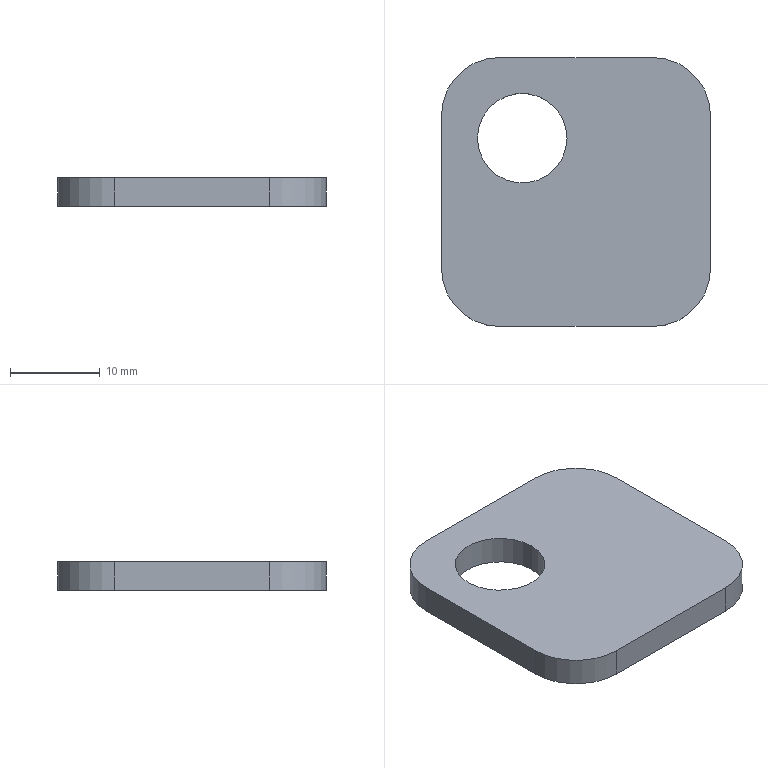Part | STEP file | [04]-6 | 1 solid | 12 faces | box 30 x 30 x 3.2 mm | volume 2516 mm3 | cylinder 6 | plane 6 | commonest cylinder face diameters 12.8 x4 10 x2
STEP:
#1=CARTESIAN_POINT('',(4.,21.,0.));
#2=VERTEX_POINT('',#1);
#3=CARTESIAN_POINT('',(14.,21.,0.));
#4=VERTEX_POINT('',#3);
#5=CARTESIAN_POINT('',(9.,21.,0.));
#6=DIRECTION('',(0.,0.,1.));
#7=DIRECTION('',(1.,0.,0.));
#8=AXIS2_PLACEMENT_3D('',#5,#6,#7);
#9=CIRCLE('',#8,5.);
#10=EDGE_CURVE('',#2,#4,#9,.T.);
#11=ORIENTED_EDGE('',*,*,#10,.F.);
#12=CARTESIAN_POINT('',(4.,21.,3.2));
#13=VERTEX_POINT('',#12);
#14=CARTESIAN_POINT('',(4.,21.,0.));
#15=DIRECTION('',(0.,0.,1.));
#16=VECTOR('',#15,1000.);
#17=LINE('',#14,#16);
#18=EDGE_CURVE('',#2,#13,#17,.T.);
#19=ORIENTED_EDGE('',*,*,#18,.T.);
#20=CARTESIAN_POINT('',(14.,21.,3.2));
#21=VERTEX_POINT('',#20);
#22=CARTESIAN_POINT('',(9.,21.,3.2));
#23=DIRECTION('',(0.,0.,-1.));
#24=DIRECTION('',(-1.,0.,0.));
#25=AXIS2_PLACEMENT_3D('',#22,#23,#24);
#26=CIRCLE('',#25,5.);
#27=EDGE_CURVE('',#21,#13,#26,.T.);
#28=ORIENTED_EDGE('',*,*,#27,.F.);
#29=CARTESIAN_POINT('',(14.,21.,0.));
#30=DIRECTION('',(0.,0.,1.));
#31=VECTOR('',#30,1000.);
#32=LINE('',#29,#31);
#33=EDGE_CURVE('',#4,#21,#32,.T.);
#34=ORIENTED_EDGE('',*,*,#33,.F.);
#35=EDGE_LOOP('',(#11,#19,#28,#34));
#36=FACE_OUTER_BOUND('',#35,.T.);
#37=CARTESIAN_POINT('',(9.,21.,0.));
#38=DIRECTION('',(0.,0.,1.));
#39=DIRECTION('',(1.,0.,0.));
#40=AXIS2_PLACEMENT_3D('',#37,#38,#39);
#41=CYLINDRICAL_SURFACE('',#40,5.);
#42=ADVANCED_FACE('',(#36),#41,.F.);
#43=ORIENTED_EDGE('',*,*,#27,.T.);
#44=CARTESIAN_POINT('',(9.,21.,3.2));
#45=DIRECTION('',(0.,0.,-1.));
#46=DIRECTION('',(-1.,0.,0.));
#47=AXIS2_PLACEMENT_3D('',#44,#45,#46);
#48=CIRCLE('',#47,5.);
#49=EDGE_CURVE('',#13,#21,#48,.T.);
#50=ORIENTED_EDGE('',*,*,#49,.T.);
#51=EDGE_LOOP('',(#43,#50));
#52=FACE_BOUND('',#51,.T.);
#53=CARTESIAN_POINT('',(30.,23.6,3.2));
#54=VERTEX_POINT('',#53);
#55=CARTESIAN_POINT('',(30.,6.4,3.2));
#56=VERTEX_POINT('',#55);
#57=CARTESIAN_POINT('',(30.,15.,3.2));
#58=DIRECTION('',(0.,-1.,0.));
#59=VECTOR('',#58,1000.);
#60=LINE('',#57,#59);
#61=EDGE_CURVE('',#54,#56,#60,.T.);
#62=ORIENTED_EDGE('',*,*,#61,.F.);
#63=CARTESIAN_POINT('',(23.6,30.,3.2));
#64=VERTEX_POINT('',#63);
#65=CARTESIAN_POINT('',(23.6,23.6,3.2));
#66=DIRECTION('',(0.,0.,1.));
#67=DIRECTION('',(1.,0.,0.));
#68=AXIS2_PLACEMENT_3D('',#65,#66,#67);
#69=CIRCLE('',#68,6.4);
#70=EDGE_CURVE('',#54,#64,#69,.T.);
#71=ORIENTED_EDGE('',*,*,#70,.T.);
#72=CARTESIAN_POINT('',(6.4,30.,3.2));
#73=VERTEX_POINT('',#72);
#74=CARTESIAN_POINT('',(15.,30.,3.2));
#75=DIRECTION('',(1.,0.,0.));
#76=VECTOR('',#75,1000.);
#77=LINE('',#74,#76);
#78=EDGE_CURVE('',#73,#64,#77,.T.);
#79=ORIENTED_EDGE('',*,*,#78,.F.);
#80=CARTESIAN_POINT('',(0.,23.6,3.2));
#81=VERTEX_POINT('',#80);
#82=CARTESIAN_POINT('',(6.4,23.6,3.2));
#83=DIRECTION('',(0.,0.,1.));
#84=DIRECTION('',(1.,0.,0.));
#85=AXIS2_PLACEMENT_3D('',#82,#83,#84);
#86=CIRCLE('',#85,6.4);
#87=EDGE_CURVE('',#73,#81,#86,.T.);
#88=ORIENTED_EDGE('',*,*,#87,.T.);
#89=CARTESIAN_POINT('',(0.,6.4,3.2));
#90=VERTEX_POINT('',#89);
#91=CARTESIAN_POINT('',(0.,15.,3.2));
#92=DIRECTION('',(0.,1.,0.));
#93=VECTOR('',#92,1000.);
#94=LINE('',#91,#93);
#95=EDGE_CURVE('',#90,#81,#94,.T.);
#96=ORIENTED_EDGE('',*,*,#95,.F.);
#97=CARTESIAN_POINT('',(6.4,0.,3.2));
#98=VERTEX_POINT('',#97);
#99=CARTESIAN_POINT('',(6.4,6.4,3.2));
#100=DIRECTION('',(0.,0.,1.));
#101=DIRECTION('',(1.,0.,0.));
#102=AXIS2_PLACEMENT_3D('',#99,#100,#101);
#103=CIRCLE('',#102,6.4);
#104=EDGE_CURVE('',#90,#98,#103,.T.);
#105=ORIENTED_EDGE('',*,*,#104,.T.);
#106=CARTESIAN_POINT('',(23.6,0.,3.2));
#107=VERTEX_POINT('',#106);
#108=CARTESIAN_POINT('',(15.,0.,3.2));
#109=DIRECTION('',(-1.,0.,0.));
#110=VECTOR('',#109,1000.);
#111=LINE('',#108,#110);
#112=EDGE_CURVE('',#107,#98,#111,.T.);
#113=ORIENTED_EDGE('',*,*,#112,.F.);
#114=CARTESIAN_POINT('',(23.6,6.4,3.2));
#115=DIRECTION('',(0.,0.,1.));
#116=DIRECTION('',(1.,0.,0.));
#117=AXIS2_PLACEMENT_3D('',#114,#115,#116);
#118=CIRCLE('',#117,6.4);
#119=EDGE_CURVE('',#107,#56,#118,.T.);
#120=ORIENTED_EDGE('',*,*,#119,.T.);
#121=EDGE_LOOP('',(#62,#71,#79,#88,#96,#105,#113,#120));
#122=FACE_OUTER_BOUND('',#121,.T.);
#123=CARTESIAN_POINT('',(15.,15.,3.2));
#124=DIRECTION('',(0.,0.,1.));
#125=DIRECTION('',(1.,0.,0.));
#126=AXIS2_PLACEMENT_3D('',#123,#124,#125);
#127=PLANE('',#126);
#128=ADVANCED_FACE('',(#52,#122),#127,.T.);
#129=CARTESIAN_POINT('',(6.4,0.,0.));
#130=VERTEX_POINT('',#129);
#131=CARTESIAN_POINT('',(23.6,0.,0.));
#132=VERTEX_POINT('',#131);
#133=CARTESIAN_POINT('',(15.,0.,0.));
#134=DIRECTION('',(1.,0.,0.));
#135=VECTOR('',#134,1000.);
#136=LINE('',#133,#135);
#137=EDGE_CURVE('',#130,#132,#136,.T.);
#138=ORIENTED_EDGE('',*,*,#137,.T.);
#139=CARTESIAN_POINT('',(23.6,0.,0.));
#140=DIRECTION('',(0.,0.,1.));
#141=VECTOR('',#140,1000.);
#142=LINE('',#139,#141);
#143=EDGE_CURVE('',#132,#107,#142,.T.);
#144=ORIENTED_EDGE('',*,*,#143,.T.);
#145=ORIENTED_EDGE('',*,*,#112,.T.);
#146=CARTESIAN_POINT('',(6.4,0.,0.));
#147=DIRECTION('',(0.,0.,-1.));
#148=VECTOR('',#147,1000.);
#149=LINE('',#146,#148);
#150=EDGE_CURVE('',#98,#130,#149,.T.);
#151=ORIENTED_EDGE('',*,*,#150,.T.);
#152=EDGE_LOOP('',(#138,#144,#145,#151));
#153=FACE_OUTER_BOUND('',#152,.T.);
#154=CARTESIAN_POINT('',(15.,0.,0.));
#155=DIRECTION('',(0.,-1.,0.));
#156=DIRECTION('',(0.,0.,-1.));
#157=AXIS2_PLACEMENT_3D('',#154,#155,#156);
#158=PLANE('',#157);
#159=ADVANCED_FACE('',(#153),#158,.T.);
#160=ORIENTED_EDGE('',*,*,#95,.T.);
#161=CARTESIAN_POINT('',(0.,23.6,0.));
#162=VERTEX_POINT('',#161);
#163=CARTESIAN_POINT('',(0.,23.6,0.));
#164=DIRECTION('',(0.,0.,-1.));
#165=VECTOR('',#164,1000.);
#166=LINE('',#163,#165);
#167=EDGE_CURVE('',#81,#162,#166,.T.);
#168=ORIENTED_EDGE('',*,*,#167,.T.);
#169=CARTESIAN_POINT('',(0.,6.4,0.));
#170=VERTEX_POINT('',#169);
#171=CARTESIAN_POINT('',(0.,15.,0.));
#172=DIRECTION('',(0.,-1.,0.));
#173=VECTOR('',#172,1000.);
#174=LINE('',#171,#173);
#175=EDGE_CURVE('',#162,#170,#174,.T.);
#176=ORIENTED_EDGE('',*,*,#175,.T.);
#177=CARTESIAN_POINT('',(0.,6.4,0.));
#178=DIRECTION('',(0.,0.,1.));
#179=VECTOR('',#178,1000.);
#180=LINE('',#177,#179);
#181=EDGE_CURVE('',#170,#90,#180,.T.);
#182=ORIENTED_EDGE('',*,*,#181,.T.);
#183=EDGE_LOOP('',(#160,#168,#176,#182));
#184=FACE_OUTER_BOUND('',#183,.T.);
#185=CARTESIAN_POINT('',(0.,15.,0.));
#186=DIRECTION('',(-1.,0.,0.));
#187=DIRECTION('',(0.,0.,1.));
#188=AXIS2_PLACEMENT_3D('',#185,#186,#187);
#189=PLANE('',#188);
#190=ADVANCED_FACE('',(#184),#189,.T.);
#191=ORIENTED_EDGE('',*,*,#78,.T.);
#192=CARTESIAN_POINT('',(23.6,30.,0.));
#193=VERTEX_POINT('',#192);
#194=CARTESIAN_POINT('',(23.6,30.,0.));
#195=DIRECTION('',(0.,0.,-1.));
#196=VECTOR('',#195,1000.);
#197=LINE('',#194,#196);
#198=EDGE_CURVE('',#64,#193,#197,.T.);
#199=ORIENTED_EDGE('',*,*,#198,.T.);
#200=CARTESIAN_POINT('',(6.4,30.,0.));
#201=VERTEX_POINT('',#200);
#202=CARTESIAN_POINT('',(15.,30.,0.));
#203=DIRECTION('',(-1.,0.,0.));
#204=VECTOR('',#203,1000.);
#205=LINE('',#202,#204);
#206=EDGE_CURVE('',#193,#201,#205,.T.);
#207=ORIENTED_EDGE('',*,*,#206,.T.);
#208=CARTESIAN_POINT('',(6.4,30.,0.));
#209=DIRECTION('',(0.,0.,1.));
#210=VECTOR('',#209,1000.);
#211=LINE('',#208,#210);
#212=EDGE_CURVE('',#201,#73,#211,.T.);
#213=ORIENTED_EDGE('',*,*,#212,.T.);
#214=EDGE_LOOP('',(#191,#199,#207,#213));
#215=FACE_OUTER_BOUND('',#214,.T.);
#216=CARTESIAN_POINT('',(15.,30.,0.));
#217=DIRECTION('',(0.,1.,0.));
#218=DIRECTION('',(0.,0.,1.));
#219=AXIS2_PLACEMENT_3D('',#216,#217,#218);
#220=PLANE('',#219);
#221=ADVANCED_FACE('',(#215),#220,.T.);
#222=CARTESIAN_POINT('',(9.,21.,0.));
#223=DIRECTION('',(0.,0.,1.));
#224=DIRECTION('',(1.,0.,0.));
#225=AXIS2_PLACEMENT_3D('',#222,#223,#224);
#226=CIRCLE('',#225,5.);
#227=EDGE_CURVE('',#4,#2,#226,.T.);
#228=ORIENTED_EDGE('',*,*,#227,.T.);
#229=ORIENTED_EDGE('',*,*,#10,.T.);
#230=EDGE_LOOP('',(#228,#229));
#231=FACE_BOUND('',#230,.T.);
#232=ORIENTED_EDGE('',*,*,#206,.F.);
#233=CARTESIAN_POINT('',(30.,23.6,0.));
#234=VERTEX_POINT('',#233);
#235=CARTESIAN_POINT('',(23.6,23.6,0.));
#236=DIRECTION('',(0.,0.,-1.));
#237=DIRECTION('',(-1.,0.,0.));
#238=AXIS2_PLACEMENT_3D('',#235,#236,#237);
#239=CIRCLE('',#238,6.4);
#240=EDGE_CURVE('',#193,#234,#239,.T.);
#241=ORIENTED_EDGE('',*,*,#240,.T.);
#242=CARTESIAN_POINT('',(30.,6.4,0.));
#243=VERTEX_POINT('',#242);
#244=CARTESIAN_POINT('',(30.,15.,0.));
#245=DIRECTION('',(0.,1.,0.));
#246=VECTOR('',#245,1000.);
#247=LINE('',#244,#246);
#248=EDGE_CURVE('',#243,#234,#247,.T.);
#249=ORIENTED_EDGE('',*,*,#248,.F.);
#250=CARTESIAN_POINT('',(23.6,6.4,0.));
#251=DIRECTION('',(0.,0.,-1.));
#252=DIRECTION('',(-1.,0.,0.));
#253=AXIS2_PLACEMENT_3D('',#250,#251,#252);
#254=CIRCLE('',#253,6.4);
#255=EDGE_CURVE('',#243,#132,#254,.T.);
#256=ORIENTED_EDGE('',*,*,#255,.T.);
#257=ORIENTED_EDGE('',*,*,#137,.F.);
#258=CARTESIAN_POINT('',(6.4,6.4,0.));
#259=DIRECTION('',(0.,0.,-1.));
#260=DIRECTION('',(-1.,0.,0.));
#261=AXIS2_PLACEMENT_3D('',#258,#259,#260);
#262=CIRCLE('',#261,6.4);
#263=EDGE_CURVE('',#130,#170,#262,.T.);
#264=ORIENTED_EDGE('',*,*,#263,.T.);
#265=ORIENTED_EDGE('',*,*,#175,.F.);
#266=CARTESIAN_POINT('',(6.4,23.6,0.));
#267=DIRECTION('',(0.,0.,-1.));
#268=DIRECTION('',(-1.,0.,0.));
#269=AXIS2_PLACEMENT_3D('',#266,#267,#268);
#270=CIRCLE('',#269,6.4);
#271=EDGE_CURVE('',#162,#201,#270,.T.);
#272=ORIENTED_EDGE('',*,*,#271,.T.);
#273=EDGE_LOOP('',(#232,#241,#249,#256,#257,#264,#265,#272));
#274=FACE_OUTER_BOUND('',#273,.T.);
#275=CARTESIAN_POINT('',(15.,15.,0.));
#276=DIRECTION('',(0.,0.,-1.));
#277=DIRECTION('',(-1.,0.,0.));
#278=AXIS2_PLACEMENT_3D('',#275,#276,#277);
#279=PLANE('',#278);
#280=ADVANCED_FACE('',(#231,#274),#279,.T.);
#281=ORIENTED_EDGE('',*,*,#248,.T.);
#282=CARTESIAN_POINT('',(30.,23.6,0.));
#283=DIRECTION('',(0.,0.,1.));
#284=VECTOR('',#283,1000.);
#285=LINE('',#282,#284);
#286=EDGE_CURVE('',#234,#54,#285,.T.);
#287=ORIENTED_EDGE('',*,*,#286,.T.);
#288=ORIENTED_EDGE('',*,*,#61,.T.);
#289=CARTESIAN_POINT('',(30.,6.4,0.));
#290=DIRECTION('',(0.,0.,-1.));
#291=VECTOR('',#290,1000.);
#292=LINE('',#289,#291);
#293=EDGE_CURVE('',#56,#243,#292,.T.);
#294=ORIENTED_EDGE('',*,*,#293,.T.);
#295=EDGE_LOOP('',(#281,#287,#288,#294));
#296=FACE_OUTER_BOUND('',#295,.T.);
#297=CARTESIAN_POINT('',(30.,15.,0.));
#298=DIRECTION('',(1.,0.,0.));
#299=DIRECTION('',(0.,0.,-1.));
#300=AXIS2_PLACEMENT_3D('',#297,#298,#299);
#301=PLANE('',#300);
#302=ADVANCED_FACE('',(#296),#301,.T.);
#303=ORIENTED_EDGE('',*,*,#263,.F.);
#304=ORIENTED_EDGE('',*,*,#150,.F.);
#305=ORIENTED_EDGE('',*,*,#104,.F.);
#306=ORIENTED_EDGE('',*,*,#181,.F.);
#307=EDGE_LOOP('',(#303,#304,#305,#306));
#308=FACE_OUTER_BOUND('',#307,.T.);
#309=CARTESIAN_POINT('',(6.4,6.4,0.));
#310=DIRECTION('',(0.,0.,1.));
#311=DIRECTION('',(1.,0.,0.));
#312=AXIS2_PLACEMENT_3D('',#309,#310,#311);
#313=CYLINDRICAL_SURFACE('',#312,6.4);
#314=ADVANCED_FACE('',(#308),#313,.T.);
#315=ORIENTED_EDGE('',*,*,#255,.F.);
#316=ORIENTED_EDGE('',*,*,#293,.F.);
#317=ORIENTED_EDGE('',*,*,#119,.F.);
#318=ORIENTED_EDGE('',*,*,#143,.F.);
#319=EDGE_LOOP('',(#315,#316,#317,#318));
#320=FACE_OUTER_BOUND('',#319,.T.);
#321=CARTESIAN_POINT('',(23.6,6.4,0.));
#322=DIRECTION('',(0.,0.,1.));
#323=DIRECTION('',(1.,0.,0.));
#324=AXIS2_PLACEMENT_3D('',#321,#322,#323);
#325=CYLINDRICAL_SURFACE('',#324,6.4);
#326=ADVANCED_FACE('',(#320),#325,.T.);
#327=ORIENTED_EDGE('',*,*,#271,.F.);
#328=ORIENTED_EDGE('',*,*,#167,.F.);
#329=ORIENTED_EDGE('',*,*,#87,.F.);
#330=ORIENTED_EDGE('',*,*,#212,.F.);
#331=EDGE_LOOP('',(#327,#328,#329,#330));
#332=FACE_OUTER_BOUND('',#331,.T.);
#333=CARTESIAN_POINT('',(6.4,23.6,0.));
#334=DIRECTION('',(0.,0.,1.));
#335=DIRECTION('',(1.,0.,0.));
#336=AXIS2_PLACEMENT_3D('',#333,#334,#335);
#337=CYLINDRICAL_SURFACE('',#336,6.4);
#338=ADVANCED_FACE('',(#332),#337,.T.);
#339=ORIENTED_EDGE('',*,*,#240,.F.);
#340=ORIENTED_EDGE('',*,*,#198,.F.);
#341=ORIENTED_EDGE('',*,*,#70,.F.);
#342=ORIENTED_EDGE('',*,*,#286,.F.);
#343=EDGE_LOOP('',(#339,#340,#341,#342));
#344=FACE_OUTER_BOUND('',#343,.T.);
#345=CARTESIAN_POINT('',(23.6,23.6,0.));
#346=DIRECTION('',(0.,0.,1.));
#347=DIRECTION('',(1.,0.,0.));
#348=AXIS2_PLACEMENT_3D('',#345,#346,#347);
#349=CYLINDRICAL_SURFACE('',#348,6.4);
#350=ADVANCED_FACE('',(#344),#349,.T.);
#351=ORIENTED_EDGE('',*,*,#18,.F.);
#352=ORIENTED_EDGE('',*,*,#227,.F.);
#353=ORIENTED_EDGE('',*,*,#33,.T.);
#354=ORIENTED_EDGE('',*,*,#49,.F.);
#355=EDGE_LOOP('',(#351,#352,#353,#354));
#356=FACE_OUTER_BOUND('',#355,.T.);
#357=CARTESIAN_POINT('',(9.,21.,0.));
#358=DIRECTION('',(0.,0.,1.));
#359=DIRECTION('',(1.,0.,0.));
#360=AXIS2_PLACEMENT_3D('',#357,#358,#359);
#361=CYLINDRICAL_SURFACE('',#360,5.);
#362=ADVANCED_FACE('',(#356),#361,.F.);
#363=CLOSED_SHELL('',(#42,#128,#159,#190,#221,#280,#302,#314,#326,#338,#350,#362));
#364=MANIFOLD_SOLID_BREP('',#363);
#365=CARTESIAN_POINT('',(0.,0.,0.));
#366=DIRECTION('',(0.,0.,1.));
#367=DIRECTION('',(1.,0.,0.));
#368=AXIS2_PLACEMENT_3D('',#365,#366,#367);
#369=(LENGTH_UNIT()NAMED_UNIT(*)SI_UNIT(.MILLI.,.METRE.));
#370=UNCERTAINTY_MEASURE_WITH_UNIT(LENGTH_MEASURE(0.00001),#369,'','');
#371=(NAMED_UNIT(*)PLANE_ANGLE_UNIT()SI_UNIT($,.RADIAN.));
#372=(NAMED_UNIT(*)SI_UNIT($,.STERADIAN.)SOLID_ANGLE_UNIT());
#373=(GEOMETRIC_REPRESENTATION_CONTEXT(3)GLOBAL_UNCERTAINTY_ASSIGNED_CONTEXT((#370))GLOBAL_UNIT_ASSIGNED_CONTEXT((#369,#371,#372))REPRESENTATION_CONTEXT('',''));
#374=ADVANCED_BREP_SHAPE_REPRESENTATION('',(#364,#368),#373);